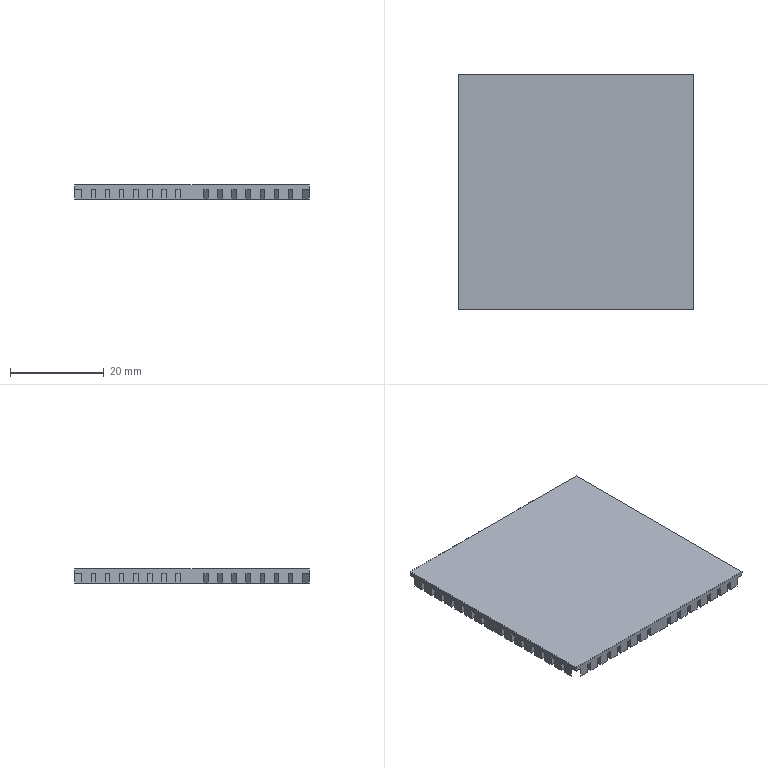Part | SolidWorks | features ICE 2, Extrusion 1 | 1 solid | 234 faces | box 50 x 50 x 3 mm | volume 5676 mm3 | plane 234